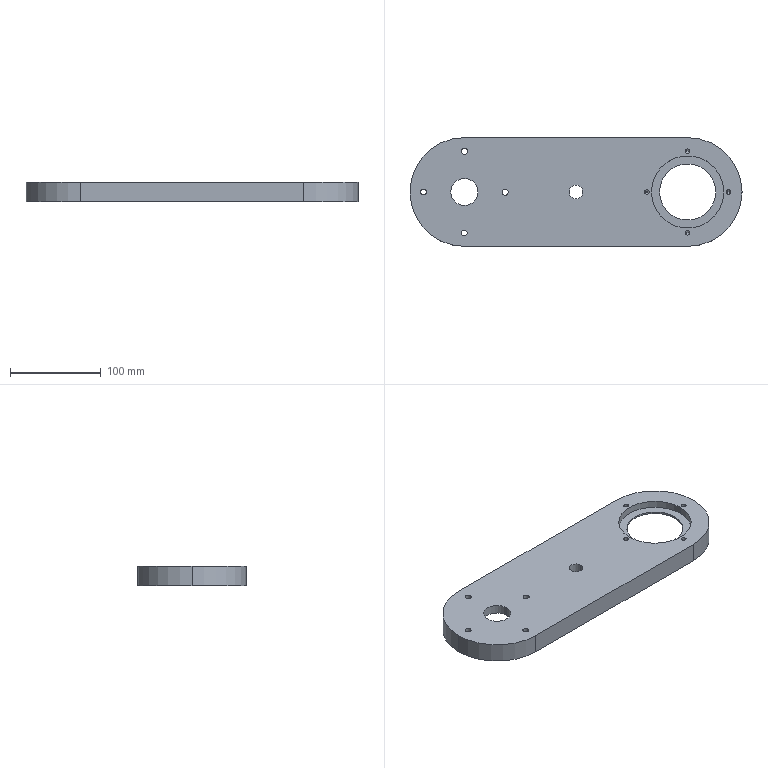Part | STEP file | Twist pulley housing SGN-4-03 | 1 solid | 66 faces | box 366.38 x 120 x 22 mm | volume 577350 mm3 | cylinder 39 | cone 16 | plane 11 | commonest cylinder face diameters 5 x8 6.6 x8 10 x6 106 x6 120 x3 15 x2